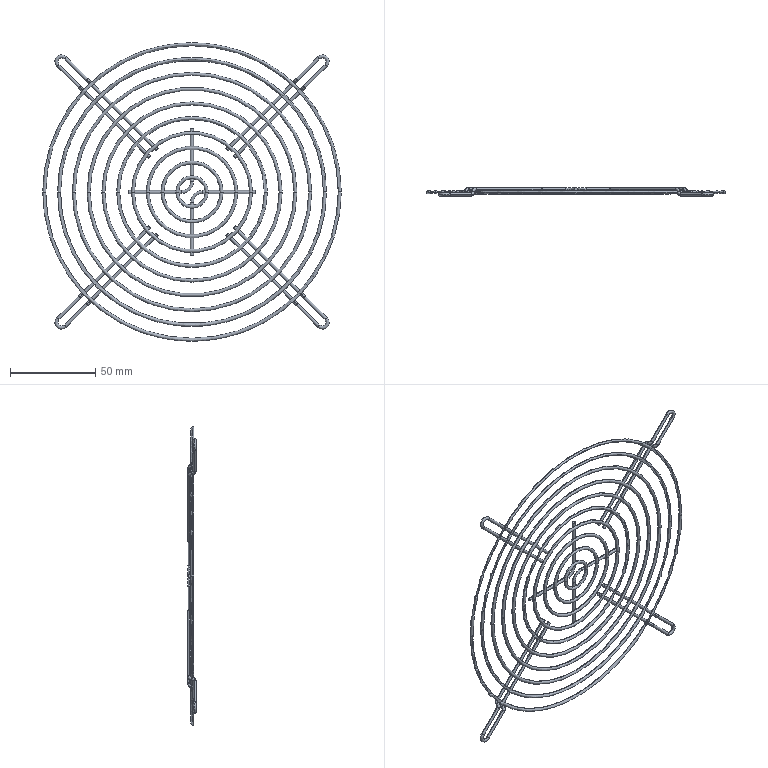Part | STEP file | 001-001-TX180 metal mesh cover[TX180]_TX180 | 16 solids | 152 faces | box 175 x 5 x 175 mm | volume 9660 mm3 | torus 84 | cylinder 56 | plane 12 | commonest cylinder face diameters 1.8 x56